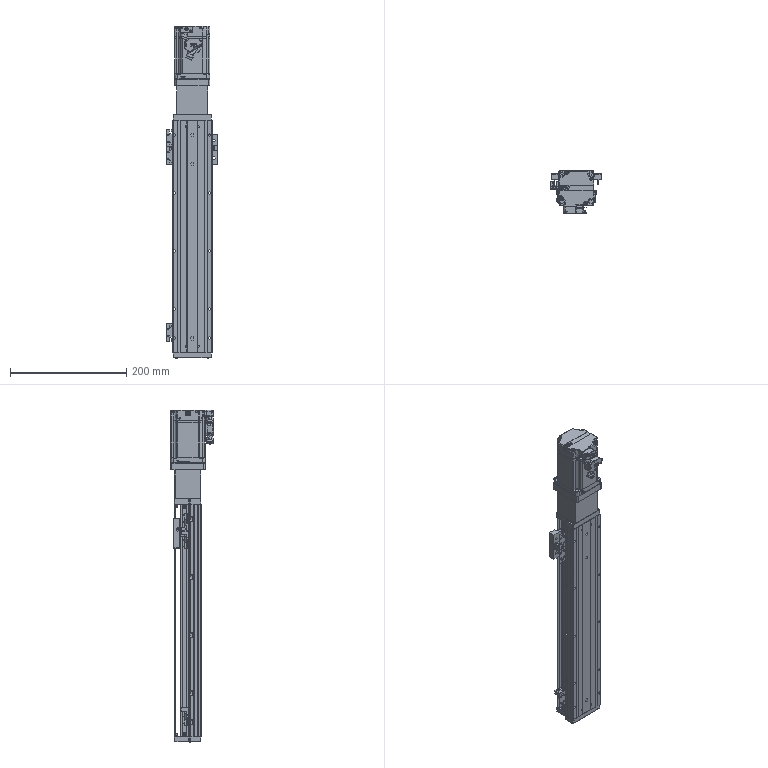Part | SolidWorks | 40 solids | 2788 faces | plane 1365 | cylinder 787 | cone 315 | spline 297 | torus 24 | commonest cylinder face diameters 2 x116 1 x104 4 x88 2.5 x50 5.5 x39 3 x34